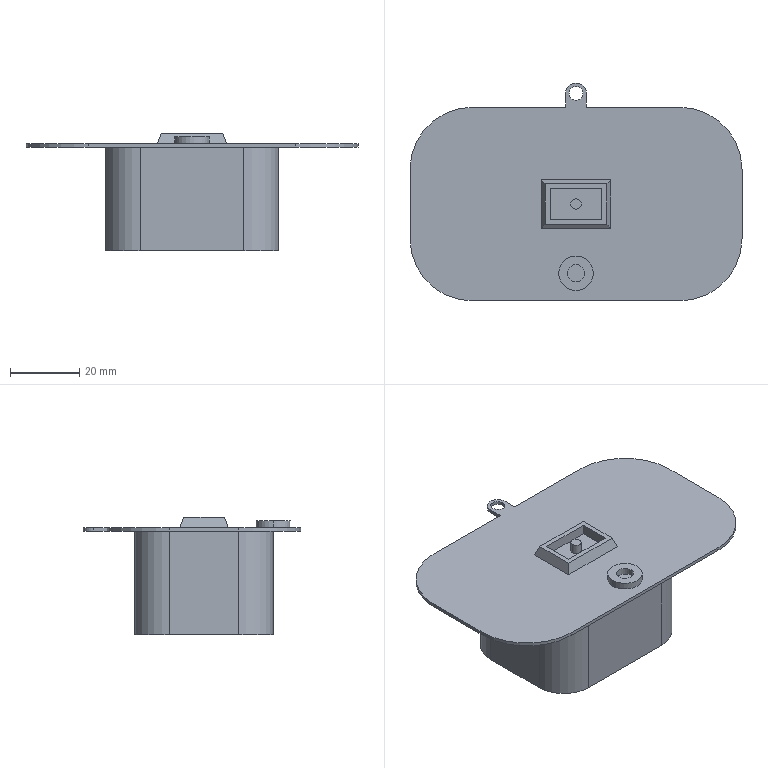Part | SolidWorks | features ICE 4, Fillet 2, Extrusion 1 | 1 solid | 53 faces | box 96 x 63 x 34 mm | volume 14984 mm3 | plane 32 | cylinder 21 | commonest cylinder face diameters 16 x4 20 x4 36 x4 3 x2 4 x2 5 x2
STEP:
#1=CARTESIAN_POINT('',(-2.5,-20.,3.));
#2=VERTEX_POINT('',#1);
#3=CARTESIAN_POINT('',(2.5,-20.,3.));
#4=VERTEX_POINT('',#3);
#5=CARTESIAN_POINT('',(0.,-20.,3.));
#6=DIRECTION('',(0.,0.,1.));
#7=DIRECTION('',(1.,0.,0.));
#8=AXIS2_PLACEMENT_3D('',#5,#6,#7);
#9=CIRCLE('',#8,2.5);
#10=EDGE_CURVE('',#2,#4,#9,.T.);
#11=ORIENTED_EDGE('',*,*,#10,.T.);
#12=CARTESIAN_POINT('',(2.5,-20.,1.));
#13=VERTEX_POINT('',#12);
#14=CARTESIAN_POINT('',(2.5,-20.,3.));
#15=DIRECTION('',(0.,0.,-1.));
#16=VECTOR('',#15,1000.);
#17=LINE('',#14,#16);
#18=EDGE_CURVE('',#4,#13,#17,.T.);
#19=ORIENTED_EDGE('',*,*,#18,.T.);
#20=CARTESIAN_POINT('',(-2.5,-20.,1.));
#21=VERTEX_POINT('',#20);
#22=CARTESIAN_POINT('',(0.,-20.,1.));
#23=DIRECTION('',(0.,0.,-1.));
#24=DIRECTION('',(1.,0.,0.));
#25=AXIS2_PLACEMENT_3D('',#22,#23,#24);
#26=CIRCLE('',#25,2.5);
#27=EDGE_CURVE('',#13,#21,#26,.T.);
#28=ORIENTED_EDGE('',*,*,#27,.T.);
#29=CARTESIAN_POINT('',(-2.5,-20.,3.));
#30=DIRECTION('',(0.,0.,-1.));
#31=VECTOR('',#30,1000.);
#32=LINE('',#29,#31);
#33=EDGE_CURVE('',#2,#21,#32,.T.);
#34=ORIENTED_EDGE('',*,*,#33,.F.);
#35=EDGE_LOOP('',(#11,#19,#28,#34));
#36=FACE_OUTER_BOUND('',#35,.T.);
#37=CARTESIAN_POINT('',(0.,-20.,3.));
#38=DIRECTION('',(0.,0.,-1.));
#39=DIRECTION('',(-1.,0.,0.));
#40=AXIS2_PLACEMENT_3D('',#37,#38,#39);
#41=CYLINDRICAL_SURFACE('',#40,2.5);
#42=ADVANCED_FACE('',(#36),#41,.F.);
#43=CARTESIAN_POINT('',(5.,-20.,3.));
#44=VERTEX_POINT('',#43);
#45=CARTESIAN_POINT('',(-5.,-20.,3.));
#46=VERTEX_POINT('',#45);
#47=CARTESIAN_POINT('',(0.,-20.,3.));
#48=DIRECTION('',(0.,0.,1.));
#49=DIRECTION('',(1.,0.,0.));
#50=AXIS2_PLACEMENT_3D('',#47,#48,#49);
#51=CIRCLE('',#50,5.);
#52=EDGE_CURVE('',#44,#46,#51,.T.);
#53=ORIENTED_EDGE('',*,*,#52,.F.);
#54=CARTESIAN_POINT('',(5.,-20.,1.));
#55=VERTEX_POINT('',#54);
#56=CARTESIAN_POINT('',(5.,-20.,3.));
#57=DIRECTION('',(0.,0.,-1.));
#58=VECTOR('',#57,1000.);
#59=LINE('',#56,#58);
#60=EDGE_CURVE('',#44,#55,#59,.T.);
#61=ORIENTED_EDGE('',*,*,#60,.T.);
#62=CARTESIAN_POINT('',(-5.,-20.,1.));
#63=VERTEX_POINT('',#62);
#64=CARTESIAN_POINT('',(0.,-20.,1.));
#65=DIRECTION('',(0.,0.,1.));
#66=DIRECTION('',(1.,0.,0.));
#67=AXIS2_PLACEMENT_3D('',#64,#65,#66);
#68=CIRCLE('',#67,5.);
#69=EDGE_CURVE('',#55,#63,#68,.T.);
#70=ORIENTED_EDGE('',*,*,#69,.T.);
#71=CARTESIAN_POINT('',(-5.,-20.,3.));
#72=DIRECTION('',(0.,0.,-1.));
#73=VECTOR('',#72,1000.);
#74=LINE('',#71,#73);
#75=EDGE_CURVE('',#46,#63,#74,.T.);
#76=ORIENTED_EDGE('',*,*,#75,.F.);
#77=EDGE_LOOP('',(#53,#61,#70,#76));
#78=FACE_OUTER_BOUND('',#77,.T.);
#79=CARTESIAN_POINT('',(0.,-20.,3.));
#80=DIRECTION('',(0.,0.,-1.));
#81=DIRECTION('',(-1.,0.,0.));
#82=AXIS2_PLACEMENT_3D('',#79,#80,#81);
#83=CYLINDRICAL_SURFACE('',#82,5.);
#84=ADVANCED_FACE('',(#78),#83,.T.);
#85=CARTESIAN_POINT('',(1.5,0.,1.));
#86=VERTEX_POINT('',#85);
#87=CARTESIAN_POINT('',(-1.5,0.,1.));
#88=VERTEX_POINT('',#87);
#89=CARTESIAN_POINT('',(0.,0.,1.));
#90=DIRECTION('',(0.,0.,1.));
#91=DIRECTION('',(1.,0.,0.));
#92=AXIS2_PLACEMENT_3D('',#89,#90,#91);
#93=CIRCLE('',#92,1.5);
#94=EDGE_CURVE('',#86,#88,#93,.T.);
#95=ORIENTED_EDGE('',*,*,#94,.T.);
#96=CARTESIAN_POINT('',(-1.5,0.,4.));
#97=VERTEX_POINT('',#96);
#98=CARTESIAN_POINT('',(-1.5,0.,1.));
#99=DIRECTION('',(0.,0.,1.));
#100=VECTOR('',#99,1000.);
#101=LINE('',#98,#100);
#102=EDGE_CURVE('',#88,#97,#101,.T.);
#103=ORIENTED_EDGE('',*,*,#102,.T.);
#104=CARTESIAN_POINT('',(1.5,0.,4.));
#105=VERTEX_POINT('',#104);
#106=CARTESIAN_POINT('',(0.,0.,4.));
#107=DIRECTION('',(0.,0.,1.));
#108=DIRECTION('',(1.,0.,0.));
#109=AXIS2_PLACEMENT_3D('',#106,#107,#108);
#110=CIRCLE('',#109,1.5);
#111=EDGE_CURVE('',#105,#97,#110,.T.);
#112=ORIENTED_EDGE('',*,*,#111,.F.);
#113=CARTESIAN_POINT('',(1.5,0.,1.));
#114=DIRECTION('',(0.,0.,1.));
#115=VECTOR('',#114,1000.);
#116=LINE('',#113,#115);
#117=EDGE_CURVE('',#86,#105,#116,.T.);
#118=ORIENTED_EDGE('',*,*,#117,.F.);
#119=EDGE_LOOP('',(#95,#103,#112,#118));
#120=FACE_OUTER_BOUND('',#119,.T.);
#121=CARTESIAN_POINT('',(0.,0.,1.));
#122=DIRECTION('',(0.,0.,1.));
#123=DIRECTION('',(1.,0.,0.));
#124=AXIS2_PLACEMENT_3D('',#121,#122,#123);
#125=CYLINDRICAL_SURFACE('',#124,1.5);
#126=ADVANCED_FACE('',(#120),#125,.T.);
#127=CARTESIAN_POINT('',(-2.,32.,1.));
#128=VERTEX_POINT('',#127);
#129=CARTESIAN_POINT('',(2.,32.,1.));
#130=VERTEX_POINT('',#129);
#131=CARTESIAN_POINT('',(0.,32.,1.));
#132=DIRECTION('',(0.,0.,1.));
#133=DIRECTION('',(1.,0.,0.));
#134=AXIS2_PLACEMENT_3D('',#131,#132,#133);
#135=CIRCLE('',#134,2.);
#136=EDGE_CURVE('',#128,#130,#135,.T.);
#137=ORIENTED_EDGE('',*,*,#136,.T.);
#138=CARTESIAN_POINT('',(2.,32.,0.));
#139=VERTEX_POINT('',#138);
#140=CARTESIAN_POINT('',(2.,32.,1.));
#141=DIRECTION('',(0.,0.,-1.));
#142=VECTOR('',#141,1000.);
#143=LINE('',#140,#142);
#144=EDGE_CURVE('',#130,#139,#143,.T.);
#145=ORIENTED_EDGE('',*,*,#144,.T.);
#146=CARTESIAN_POINT('',(-2.,32.,0.));
#147=VERTEX_POINT('',#146);
#148=CARTESIAN_POINT('',(0.,32.,0.));
#149=DIRECTION('',(0.,0.,1.));
#150=DIRECTION('',(1.,0.,0.));
#151=AXIS2_PLACEMENT_3D('',#148,#149,#150);
#152=CIRCLE('',#151,2.);
#153=EDGE_CURVE('',#147,#139,#152,.T.);
#154=ORIENTED_EDGE('',*,*,#153,.F.);
#155=CARTESIAN_POINT('',(-2.,32.,1.));
#156=DIRECTION('',(0.,0.,-1.));
#157=VECTOR('',#156,1000.);
#158=LINE('',#155,#157);
#159=EDGE_CURVE('',#128,#147,#158,.T.);
#160=ORIENTED_EDGE('',*,*,#159,.F.);
#161=EDGE_LOOP('',(#137,#145,#154,#160));
#162=FACE_OUTER_BOUND('',#161,.T.);
#163=CARTESIAN_POINT('',(0.,32.,1.));
#164=DIRECTION('',(0.,0.,-1.));
#165=DIRECTION('',(-1.,0.,0.));
#166=AXIS2_PLACEMENT_3D('',#163,#164,#165);
#167=CYLINDRICAL_SURFACE('',#166,2.);
#168=ADVANCED_FACE('',(#162),#167,.F.);
#169=CARTESIAN_POINT('',(-48.,-10.,0.));
#170=VERTEX_POINT('',#169);
#171=CARTESIAN_POINT('',(-30.,-28.,0.));
#172=VERTEX_POINT('',#171);
#173=CARTESIAN_POINT('',(-30.,-10.,0.));
#174=DIRECTION('',(0.,0.,1.));
#175=DIRECTION('',(1.,0.,0.));
#176=AXIS2_PLACEMENT_3D('',#173,#174,#175);
#177=CIRCLE('',#176,18.);
#178=EDGE_CURVE('',#170,#172,#177,.T.);
#179=ORIENTED_EDGE('',*,*,#178,.F.);
#180=CARTESIAN_POINT('',(-48.,10.,0.));
#181=VERTEX_POINT('',#180);
#182=CARTESIAN_POINT('',(-48.,10.,0.));
#183=DIRECTION('',(0.,-1.,0.));
#184=VECTOR('',#183,1000.);
#185=LINE('',#182,#184);
#186=EDGE_CURVE('',#181,#170,#185,.T.);
#187=ORIENTED_EDGE('',*,*,#186,.F.);
#188=CARTESIAN_POINT('',(-30.,28.,0.));
#189=VERTEX_POINT('',#188);
#190=CARTESIAN_POINT('',(-30.,10.,0.));
#191=DIRECTION('',(0.,0.,1.));
#192=DIRECTION('',(1.,0.,0.));
#193=AXIS2_PLACEMENT_3D('',#190,#191,#192);
#194=CIRCLE('',#193,18.);
#195=EDGE_CURVE('',#189,#181,#194,.T.);
#196=ORIENTED_EDGE('',*,*,#195,.F.);
#197=CARTESIAN_POINT('',(-3.,28.,0.));
#198=VERTEX_POINT('',#197);
#199=CARTESIAN_POINT('',(-30.,28.,0.));
#200=DIRECTION('',(-1.,0.,0.));
#201=VECTOR('',#200,1000.);
#202=LINE('',#199,#201);
#203=EDGE_CURVE('',#198,#189,#202,.T.);
#204=ORIENTED_EDGE('',*,*,#203,.F.);
#205=CARTESIAN_POINT('',(-3.,32.,0.));
#206=VERTEX_POINT('',#205);
#207=CARTESIAN_POINT('',(-3.,28.,0.));
#208=DIRECTION('',(0.,-1.,0.));
#209=VECTOR('',#208,1000.);
#210=LINE('',#207,#209);
#211=EDGE_CURVE('',#206,#198,#210,.T.);
#212=ORIENTED_EDGE('',*,*,#211,.F.);
#213=CARTESIAN_POINT('',(3.,32.,0.));
#214=VERTEX_POINT('',#213);
#215=CARTESIAN_POINT('',(0.,32.,0.));
#216=DIRECTION('',(0.,0.,1.));
#217=DIRECTION('',(-1.,0.,0.));
#218=AXIS2_PLACEMENT_3D('',#215,#216,#217);
#219=CIRCLE('',#218,3.);
#220=EDGE_CURVE('',#214,#206,#219,.T.);
#221=ORIENTED_EDGE('',*,*,#220,.F.);
#222=CARTESIAN_POINT('',(3.,28.,0.));
#223=VERTEX_POINT('',#222);
#224=CARTESIAN_POINT('',(3.,32.,0.));
#225=DIRECTION('',(0.,1.,0.));
#226=VECTOR('',#225,1000.);
#227=LINE('',#224,#226);
#228=EDGE_CURVE('',#223,#214,#227,.T.);
#229=ORIENTED_EDGE('',*,*,#228,.F.);
#230=CARTESIAN_POINT('',(30.,28.,0.));
#231=VERTEX_POINT('',#230);
#232=CARTESIAN_POINT('',(3.,28.,0.));
#233=DIRECTION('',(-1.,0.,0.));
#234=VECTOR('',#233,1000.);
#235=LINE('',#232,#234);
#236=EDGE_CURVE('',#231,#223,#235,.T.);
#237=ORIENTED_EDGE('',*,*,#236,.F.);
#238=CARTESIAN_POINT('',(48.,10.,0.));
#239=VERTEX_POINT('',#238);
#240=CARTESIAN_POINT('',(30.,10.,0.));
#241=DIRECTION('',(0.,0.,1.));
#242=DIRECTION('',(-1.,0.,0.));
#243=AXIS2_PLACEMENT_3D('',#240,#241,#242);
#244=CIRCLE('',#243,18.);
#245=EDGE_CURVE('',#239,#231,#244,.T.);
#246=ORIENTED_EDGE('',*,*,#245,.F.);
#247=CARTESIAN_POINT('',(48.,-10.,0.));
#248=VERTEX_POINT('',#247);
#249=CARTESIAN_POINT('',(48.,10.,0.));
#250=DIRECTION('',(0.,1.,0.));
#251=VECTOR('',#250,1000.);
#252=LINE('',#249,#251);
#253=EDGE_CURVE('',#248,#239,#252,.T.);
#254=ORIENTED_EDGE('',*,*,#253,.F.);
#255=CARTESIAN_POINT('',(30.,-28.,0.));
#256=VERTEX_POINT('',#255);
#257=CARTESIAN_POINT('',(30.,-10.,0.));
#258=DIRECTION('',(0.,0.,1.));
#259=DIRECTION('',(1.,0.,0.));
#260=AXIS2_PLACEMENT_3D('',#257,#258,#259);
#261=CIRCLE('',#260,18.);
#262=EDGE_CURVE('',#256,#248,#261,.T.);
#263=ORIENTED_EDGE('',*,*,#262,.F.);
#264=CARTESIAN_POINT('',(-30.,-28.,0.));
#265=DIRECTION('',(1.,0.,0.));
#266=VECTOR('',#265,1000.);
#267=LINE('',#264,#266);
#268=EDGE_CURVE('',#172,#256,#267,.T.);
#269=ORIENTED_EDGE('',*,*,#268,.F.);
#270=EDGE_LOOP('',(#179,#187,#196,#204,#212,#221,#229,#237,#246,#254,#263,#269));
#271=FACE_OUTER_BOUND('',#270,.T.);
#272=ORIENTED_EDGE('',*,*,#153,.T.);
#273=CARTESIAN_POINT('',(0.,32.,0.));
#274=DIRECTION('',(0.,0.,1.));
#275=DIRECTION('',(1.,0.,0.));
#276=AXIS2_PLACEMENT_3D('',#273,#274,#275);
#277=CIRCLE('',#276,2.);
#278=EDGE_CURVE('',#139,#147,#277,.T.);
#279=ORIENTED_EDGE('',*,*,#278,.T.);
#280=EDGE_LOOP('',(#272,#279));
#281=FACE_BOUND('',#280,.T.);
#282=CARTESIAN_POINT('',(-25.,-10.,0.));
#283=VERTEX_POINT('',#282);
#284=CARTESIAN_POINT('',(-25.,10.,0.));
#285=VERTEX_POINT('',#284);
#286=CARTESIAN_POINT('',(-25.,20.,0.));
#287=DIRECTION('',(0.,1.,0.));
#288=VECTOR('',#287,1000.);
#289=LINE('',#286,#288);
#290=EDGE_CURVE('',#283,#285,#289,.T.);
#291=ORIENTED_EDGE('',*,*,#290,.F.);
#292=CARTESIAN_POINT('',(-15.,-20.,0.));
#293=VERTEX_POINT('',#292);
#294=CARTESIAN_POINT('',(-15.,-10.,0.));
#295=DIRECTION('',(0.,0.,1.));
#296=DIRECTION('',(1.,0.,0.));
#297=AXIS2_PLACEMENT_3D('',#294,#295,#296);
#298=CIRCLE('',#297,10.);
#299=EDGE_CURVE('',#283,#293,#298,.T.);
#300=ORIENTED_EDGE('',*,*,#299,.T.);
#301=CARTESIAN_POINT('',(15.,-20.,0.));
#302=VERTEX_POINT('',#301);
#303=CARTESIAN_POINT('',(25.,-20.,0.));
#304=DIRECTION('',(-1.,0.,0.));
#305=VECTOR('',#304,1000.);
#306=LINE('',#303,#305);
#307=EDGE_CURVE('',#302,#293,#306,.T.);
#308=ORIENTED_EDGE('',*,*,#307,.F.);
#309=CARTESIAN_POINT('',(25.,-10.,0.));
#310=VERTEX_POINT('',#309);
#311=CARTESIAN_POINT('',(15.,-10.,0.));
#312=DIRECTION('',(0.,0.,1.));
#313=DIRECTION('',(1.,0.,0.));
#314=AXIS2_PLACEMENT_3D('',#311,#312,#313);
#315=CIRCLE('',#314,10.);
#316=EDGE_CURVE('',#302,#310,#315,.T.);
#317=ORIENTED_EDGE('',*,*,#316,.T.);
#318=CARTESIAN_POINT('',(25.,10.,0.));
#319=VERTEX_POINT('',#318);
#320=CARTESIAN_POINT('',(25.,20.,0.));
#321=DIRECTION('',(0.,-1.,0.));
#322=VECTOR('',#321,1000.);
#323=LINE('',#320,#322);
#324=EDGE_CURVE('',#319,#310,#323,.T.);
#325=ORIENTED_EDGE('',*,*,#324,.F.);
#326=CARTESIAN_POINT('',(15.,20.,0.));
#327=VERTEX_POINT('',#326);
#328=CARTESIAN_POINT('',(15.,10.,0.));
#329=DIRECTION('',(0.,0.,1.));
#330=DIRECTION('',(1.,0.,0.));
#331=AXIS2_PLACEMENT_3D('',#328,#329,#330);
#332=CIRCLE('',#331,10.);
#333=EDGE_CURVE('',#319,#327,#332,.T.);
#334=ORIENTED_EDGE('',*,*,#333,.T.);
#335=CARTESIAN_POINT('',(-15.,20.,0.));
#336=VERTEX_POINT('',#335);
#337=CARTESIAN_POINT('',(25.,20.,0.));
#338=DIRECTION('',(1.,0.,0.));
#339=VECTOR('',#338,1000.);
#340=LINE('',#337,#339);
#341=EDGE_CURVE('',#336,#327,#340,.T.);
#342=ORIENTED_EDGE('',*,*,#341,.F.);
#343=CARTESIAN_POINT('',(-15.,10.,0.));
#344=DIRECTION('',(0.,0.,1.));
#345=DIRECTION('',(1.,0.,0.));
#346=AXIS2_PLACEMENT_3D('',#343,#344,#345);
#347=CIRCLE('',#346,10.);
#348=EDGE_CURVE('',#336,#285,#347,.T.);
#349=ORIENTED_EDGE('',*,*,#348,.T.);
#350=EDGE_LOOP('',(#291,#300,#308,#317,#325,#334,#342,#349));
#351=FACE_BOUND('',#350,.T.);
#352=CARTESIAN_POINT('',(-30.,-10.,0.));
#353=DIRECTION('',(0.,0.,1.));
#354=DIRECTION('',(1.,0.,0.));
#355=AXIS2_PLACEMENT_3D('',#352,#353,#354);
#356=PLANE('',#355);
#357=ADVANCED_FACE('',(#271,#281,#351),#356,.F.);
#358=CARTESIAN_POINT('',(0.,-20.,1.));
#359=DIRECTION('',(0.,0.,1.));
#360=DIRECTION('',(1.,0.,0.));
#361=AXIS2_PLACEMENT_3D('',#358,#359,#360);
#362=CIRCLE('',#361,5.);
#363=EDGE_CURVE('',#63,#55,#362,.T.);
#364=ORIENTED_EDGE('',*,*,#363,.F.);
#365=ORIENTED_EDGE('',*,*,#69,.F.);
#366=EDGE_LOOP('',(#364,#365));
#367=FACE_BOUND('',#366,.T.);
#368=CARTESIAN_POINT('',(-48.,-10.,1.));
#369=VERTEX_POINT('',#368);
#370=CARTESIAN_POINT('',(-30.,-28.,1.));
#371=VERTEX_POINT('',#370);
#372=CARTESIAN_POINT('',(-30.,-10.,1.));
#373=DIRECTION('',(0.,0.,1.));
#374=DIRECTION('',(1.,0.,0.));
#375=AXIS2_PLACEMENT_3D('',#372,#373,#374);
#376=CIRCLE('',#375,18.);
#377=EDGE_CURVE('',#369,#371,#376,.T.);
#378=ORIENTED_EDGE('',*,*,#377,.T.);
#379=CARTESIAN_POINT('',(30.,-28.,1.));
#380=VERTEX_POINT('',#379);
#381=CARTESIAN_POINT('',(-30.,-28.,1.));
#382=DIRECTION('',(1.,0.,0.));
#383=VECTOR('',#382,1000.);
#384=LINE('',#381,#383);
#385=EDGE_CURVE('',#371,#380,#384,.T.);
#386=ORIENTED_EDGE('',*,*,#385,.T.);
#387=CARTESIAN_POINT('',(48.,-10.,1.));
#388=VERTEX_POINT('',#387);
#389=CARTESIAN_POINT('',(30.,-10.,1.));
#390=DIRECTION('',(0.,0.,1.));
#391=DIRECTION('',(1.,0.,0.));
#392=AXIS2_PLACEMENT_3D('',#389,#390,#391);
#393=CIRCLE('',#392,18.);
#394=EDGE_CURVE('',#380,#388,#393,.T.);
#395=ORIENTED_EDGE('',*,*,#394,.T.);
#396=CARTESIAN_POINT('',(48.,10.,1.));
#397=VERTEX_POINT('',#396);
#398=CARTESIAN_POINT('',(48.,10.,1.));
#399=DIRECTION('',(0.,1.,0.));
#400=VECTOR('',#399,1000.);
#401=LINE('',#398,#400);
#402=EDGE_CURVE('',#388,#397,#401,.T.);
#403=ORIENTED_EDGE('',*,*,#402,.T.);
#404=CARTESIAN_POINT('',(30.,28.,1.));
#405=VERTEX_POINT('',#404);
#406=CARTESIAN_POINT('',(30.,10.,1.));
#407=DIRECTION('',(0.,0.,1.));
#408=DIRECTION('',(-1.,0.,0.));
#409=AXIS2_PLACEMENT_3D('',#406,#407,#408);
#410=CIRCLE('',#409,18.);
#411=EDGE_CURVE('',#397,#405,#410,.T.);
#412=ORIENTED_EDGE('',*,*,#411,.T.);
#413=CARTESIAN_POINT('',(3.,28.,1.));
#414=VERTEX_POINT('',#413);
#415=CARTESIAN_POINT('',(3.,28.,1.));
#416=DIRECTION('',(-1.,0.,0.));
#417=VECTOR('',#416,1000.);
#418=LINE('',#415,#417);
#419=EDGE_CURVE('',#405,#414,#418,.T.);
#420=ORIENTED_EDGE('',*,*,#419,.T.);
#421=CARTESIAN_POINT('',(3.,32.,1.));
#422=VERTEX_POINT('',#421);
#423=CARTESIAN_POINT('',(3.,32.,1.));
#424=DIRECTION('',(0.,1.,0.));
#425=VECTOR('',#424,1000.);
#426=LINE('',#423,#425);
#427=EDGE_CURVE('',#414,#422,#426,.T.);
#428=ORIENTED_EDGE('',*,*,#427,.T.);
#429=CARTESIAN_POINT('',(-3.,32.,1.));
#430=VERTEX_POINT('',#429);
#431=CARTESIAN_POINT('',(0.,32.,1.));
#432=DIRECTION('',(0.,0.,1.));
#433=DIRECTION('',(-1.,0.,0.));
#434=AXIS2_PLACEMENT_3D('',#431,#432,#433);
#435=CIRCLE('',#434,3.);
#436=EDGE_CURVE('',#422,#430,#435,.T.);
#437=ORIENTED_EDGE('',*,*,#436,.T.);
#438=CARTESIAN_POINT('',(-3.,28.,1.));
#439=VERTEX_POINT('',#438);
#440=CARTESIAN_POINT('',(-3.,28.,1.));
#441=DIRECTION('',(0.,-1.,0.));
#442=VECTOR('',#441,1000.);
#443=LINE('',#440,#442);
#444=EDGE_CURVE('',#430,#439,#443,.T.);
#445=ORIENTED_EDGE('',*,*,#444,.T.);
#446=CARTESIAN_POINT('',(-30.,28.,1.));
#447=VERTEX_POINT('',#446);
#448=CARTESIAN_POINT('',(-30.,28.,1.));
#449=DIRECTION('',(-1.,0.,0.));
#450=VECTOR('',#449,1000.);
#451=LINE('',#448,#450);
#452=EDGE_CURVE('',#439,#447,#451,.T.);
#453=ORIENTED_EDGE('',*,*,#452,.T.);
#454=CARTESIAN_POINT('',(-48.,10.,1.));
#455=VERTEX_POINT('',#454);
#456=CARTESIAN_POINT('',(-30.,10.,1.));
#457=DIRECTION('',(0.,0.,1.));
#458=DIRECTION('',(1.,0.,0.));
#459=AXIS2_PLACEMENT_3D('',#456,#457,#458);
#460=CIRCLE('',#459,18.);
#461=EDGE_CURVE('',#447,#455,#460,.T.);
#462=ORIENTED_EDGE('',*,*,#461,.T.);
#463=CARTESIAN_POINT('',(-48.,10.,1.));
#464=DIRECTION('',(0.,-1.,0.));
#465=VECTOR('',#464,1000.);
#466=LINE('',#463,#465);
#467=EDGE_CURVE('',#455,#369,#466,.T.);
#468=ORIENTED_EDGE('',*,*,#467,.T.);
#469=EDGE_LOOP('',(#378,#386,#395,#403,#412,#420,#428,#437,#445,#453,#462,#468));
#470=FACE_OUTER_BOUND('',#469,.T.);
#471=ORIENTED_EDGE('',*,*,#136,.F.);
#472=CARTESIAN_POINT('',(0.,32.,1.));
#473=DIRECTION('',(0.,0.,1.));
#474=DIRECTION('',(1.,0.,0.));
#475=AXIS2_PLACEMENT_3D('',#472,#473,#474);
#476=CIRCLE('',#475,2.);
#477=EDGE_CURVE('',#130,#128,#476,.T.);
#478=ORIENTED_EDGE('',*,*,#477,.F.);
#479=EDGE_LOOP('',(#471,#478));
#480=FACE_BOUND('',#479,.T.);
#481=CARTESIAN_POINT('',(10.,7.,1.));
#482=VERTEX_POINT('',#481);
#483=CARTESIAN_POINT('',(-10.,7.,1.));
#484=VERTEX_POINT('',#483);
#485=CARTESIAN_POINT('',(-10.,7.,1.));
#486=DIRECTION('',(-1.,0.,0.));
#487=VECTOR('',#486,1000.);
#488=LINE('',#485,#487);
#489=EDGE_CURVE('',#482,#484,#488,.T.);
#490=ORIENTED_EDGE('',*,*,#489,.F.);
#491=CARTESIAN_POINT('',(10.,-7.,1.));
#492=VERTEX_POINT('',#491);
#493=CARTESIAN_POINT('',(10.,7.,1.));
#494=DIRECTION('',(0.,1.,0.));
#495=VECTOR('',#494,1000.);
#496=LINE('',#493,#495);
#497=EDGE_CURVE('',#492,#482,#496,.T.);
#498=ORIENTED_EDGE('',*,*,#497,.F.);
#499=CARTESIAN_POINT('',(-10.,-7.,1.));
#500=VERTEX_POINT('',#499);
#501=CARTESIAN_POINT('',(-10.,-7.,1.));
#502=DIRECTION('',(1.,0.,0.));
#503=VECTOR('',#502,1000.);
#504=LINE('',#501,#503);
#505=EDGE_CURVE('',#500,#492,#504,.T.);
#506=ORIENTED_EDGE('',*,*,#505,.F.);
#507=CARTESIAN_POINT('',(-10.,7.,1.));
#508=DIRECTION('',(0.,-1.,0.));
#509=VECTOR('',#508,1000.);
#510=LINE('',#507,#509);
#511=EDGE_CURVE('',#484,#500,#510,.T.);
#512=ORIENTED_EDGE('',*,*,#511,.F.);
#513=EDGE_LOOP('',(#490,#498,#506,#512));
#514=FACE_BOUND('',#513,.T.);
#515=CARTESIAN_POINT('',(-30.,-10.,1.));
#516=DIRECTION('',(0.,0.,1.));
#517=DIRECTION('',(1.,0.,0.));
#518=AXIS2_PLACEMENT_3D('',#515,#516,#517);
#519=PLANE('',#518);
#520=ADVANCED_FACE('',(#367,#470,#480,#514),#519,.T.);
#521=ORIENTED_EDGE('',*,*,#178,.T.);
#522=CARTESIAN_POINT('',(-30.,-28.,1.));
#523=DIRECTION('',(0.,0.,-1.));
#524=VECTOR('',#523,1000.);
#525=LINE('',#522,#524);
#526=EDGE_CURVE('',#371,#172,#525,.T.);
#527=ORIENTED_EDGE('',*,*,#526,.F.);
#528=ORIENTED_EDGE('',*,*,#377,.F.);
#529=CARTESIAN_POINT('',(-48.,-10.,1.));
#530=DIRECTION('',(0.,0.,-1.));
#531=VECTOR('',#530,1000.);
#532=LINE('',#529,#531);
#533=EDGE_CURVE('',#369,#170,#532,.T.);
#534=ORIENTED_EDGE('',*,*,#533,.T.);
#535=EDGE_LOOP('',(#521,#527,#528,#534));
#536=FACE_OUTER_BOUND('',#535,.T.);
#537=CARTESIAN_POINT('',(-30.,-10.,1.));
#538=DIRECTION('',(0.,0.,-1.));
#539=DIRECTION('',(-1.,0.,0.));
#540=AXIS2_PLACEMENT_3D('',#537,#538,#539);
#541=CYLINDRICAL_SURFACE('',#540,18.);
#542=ADVANCED_FACE('',(#536),#541,.T.);
#543=ORIENTED_EDGE('',*,*,#268,.T.);
#544=CARTESIAN_POINT('',(30.,-28.,1.));
#545=DIRECTION('',(0.,0.,-1.));
#546=VECTOR('',#545,1000.);
#547=LINE('',#544,#546);
#548=EDGE_CURVE('',#380,#256,#547,.T.);
#549=ORIENTED_EDGE('',*,*,#548,.F.);
#550=ORIENTED_EDGE('',*,*,#385,.F.);
#551=ORIENTED_EDGE('',*,*,#526,.T.);
#552=EDGE_LOOP('',(#543,#549,#550,#551));
#553=FACE_OUTER_BOUND('',#552,.T.);
#554=CARTESIAN_POINT('',(-30.,-28.,1.));
#555=DIRECTION('',(0.,1.,0.));
#556=DIRECTION('',(0.,0.,1.));
#557=AXIS2_PLACEMENT_3D('',#554,#555,#556);
#558=PLANE('',#557);
#559=ADVANCED_FACE('',(#553),#558,.F.);
#560=ORIENTED_EDGE('',*,*,#262,.T.);
#561=CARTESIAN_POINT('',(48.,-10.,1.));
#562=DIRECTION('',(0.,0.,-1.));
#563=VECTOR('',#562,1000.);
#564=LINE('',#561,#563);
#565=EDGE_CURVE('',#388,#248,#564,.T.);
#566=ORIENTED_EDGE('',*,*,#565,.F.);
#567=ORIENTED_EDGE('',*,*,#394,.F.);
#568=ORIENTED_EDGE('',*,*,#548,.T.);
#569=EDGE_LOOP('',(#560,#566,#567,#568));
#570=FACE_OUTER_BOUND('',#569,.T.);
#571=CARTESIAN_POINT('',(30.,-10.,1.));
#572=DIRECTION('',(0.,0.,-1.));
#573=DIRECTION('',(-1.,0.,0.));
#574=AXIS2_PLACEMENT_3D('',#571,#572,#573);
#575=CYLINDRICAL_SURFACE('',#574,18.);
#576=ADVANCED_FACE('',(#570),#575,.T.);
#577=ORIENTED_EDGE('',*,*,#253,.T.);
#578=CARTESIAN_POINT('',(48.,10.,1.));
#579=DIRECTION('',(0.,0.,-1.));
#580=VECTOR('',#579,1000.);
#581=LINE('',#578,#580);
#582=EDGE_CURVE('',#397,#239,#581,.T.);
#583=ORIENTED_EDGE('',*,*,#582,.F.);
#584=ORIENTED_EDGE('',*,*,#402,.F.);
#585=ORIENTED_EDGE('',*,*,#565,.T.);
#586=EDGE_LOOP('',(#577,#583,#584,#585));
#587=FACE_OUTER_BOUND('',#586,.T.);
#588=CARTESIAN_POINT('',(48.,10.,1.));
#589=DIRECTION('',(-1.,0.,0.));
#590=DIRECTION('',(0.,0.,1.));
#591=AXIS2_PLACEMENT_3D('',#588,#589,#590);
#592=PLANE('',#591);
#593=ADVANCED_FACE('',(#587),#592,.F.);
#594=ORIENTED_EDGE('',*,*,#245,.T.);
#595=CARTESIAN_POINT('',(30.,28.,1.));
#596=DIRECTION('',(0.,0.,-1.));
#597=VECTOR('',#596,1000.);
#598=LINE('',#595,#597);
#599=EDGE_CURVE('',#405,#231,#598,.T.);
#600=ORIENTED_EDGE('',*,*,#599,.F.);
#601=ORIENTED_EDGE('',*,*,#411,.F.);
#602=ORIENTED_EDGE('',*,*,#582,.T.);
#603=EDGE_LOOP('',(#594,#600,#601,#602));
#604=FACE_OUTER_BOUND('',#603,.T.);
#605=CARTESIAN_POINT('',(30.,10.,1.));
#606=DIRECTION('',(0.,0.,-1.));
#607=DIRECTION('',(-1.,0.,0.));
#608=AXIS2_PLACEMENT_3D('',#605,#606,#607);
#609=CYLINDRICAL_SURFACE('',#608,18.);
#610=ADVANCED_FACE('',(#604),#609,.T.);
#611=ORIENTED_EDGE('',*,*,#236,.T.);
#612=CARTESIAN_POINT('',(3.,28.,1.));
#613=DIRECTION('',(0.,0.,-1.));
#614=VECTOR('',#613,1000.);
#615=LINE('',#612,#614);
#616=EDGE_CURVE('',#414,#223,#615,.T.);
#617=ORIENTED_EDGE('',*,*,#616,.F.);
#618=ORIENTED_EDGE('',*,*,#419,.F.);
#619=ORIENTED_EDGE('',*,*,#599,.T.);
#620=EDGE_LOOP('',(#611,#617,#618,#619));
#621=FACE_OUTER_BOUND('',#620,.T.);
#622=CARTESIAN_POINT('',(3.,28.,1.));
#623=DIRECTION('',(0.,-1.,0.));
#624=DIRECTION('',(0.,0.,-1.));
#625=AXIS2_PLACEMENT_3D('',#622,#623,#624);
#626=PLANE('',#625);
#627=ADVANCED_FACE('',(#621),#626,.F.);
#628=ORIENTED_EDGE('',*,*,#228,.T.);
#629=CARTESIAN_POINT('',(3.,32.,1.));
#630=DIRECTION('',(0.,0.,-1.));
#631=VECTOR('',#630,1000.);
#632=LINE('',#629,#631);
#633=EDGE_CURVE('',#422,#214,#632,.T.);
#634=ORIENTED_EDGE('',*,*,#633,.F.);
#635=ORIENTED_EDGE('',*,*,#427,.F.);
#636=ORIENTED_EDGE('',*,*,#616,.T.);
#637=EDGE_LOOP('',(#628,#634,#635,#636));
#638=FACE_OUTER_BOUND('',#637,.T.);
#639=CARTESIAN_POINT('',(3.,32.,1.));
#640=DIRECTION('',(-1.,0.,0.));
#641=DIRECTION('',(0.,0.,1.));
#642=AXIS2_PLACEMENT_3D('',#639,#640,#641);
#643=PLANE('',#642);
#644=ADVANCED_FACE('',(#638),#643,.F.);
#645=ORIENTED_EDGE('',*,*,#220,.T.);
#646=CARTESIAN_POINT('',(-3.,32.,1.));
#647=DIRECTION('',(0.,0.,-1.));
#648=VECTOR('',#647,1000.);
#649=LINE('',#646,#648);
#650=EDGE_CURVE('',#430,#206,#649,.T.);
#651=ORIENTED_EDGE('',*,*,#650,.F.);
#652=ORIENTED_EDGE('',*,*,#436,.F.);
#653=ORIENTED_EDGE('',*,*,#633,.T.);
#654=EDGE_LOOP('',(#645,#651,#652,#653));
#655=FACE_OUTER_BOUND('',#654,.T.);
#656=CARTESIAN_POINT('',(0.,32.,1.));
#657=DIRECTION('',(0.,0.,-1.));
#658=DIRECTION('',(-1.,0.,0.));
#659=AXIS2_PLACEMENT_3D('',#656,#657,#658);
#660=CYLINDRICAL_SURFACE('',#659,3.);
#661=ADVANCED_FACE('',(#655),#660,.T.);
#662=ORIENTED_EDGE('',*,*,#211,.T.);
#663=CARTESIAN_POINT('',(-3.,28.,1.));
#664=DIRECTION('',(0.,0.,-1.));
#665=VECTOR('',#664,1000.);
#666=LINE('',#663,#665);
#667=EDGE_CURVE('',#439,#198,#666,.T.);
#668=ORIENTED_EDGE('',*,*,#667,.F.);
#669=ORIENTED_EDGE('',*,*,#444,.F.);
#670=ORIENTED_EDGE('',*,*,#650,.T.);
#671=EDGE_LOOP('',(#662,#668,#669,#670));
#672=FACE_OUTER_BOUND('',#671,.T.);
#673=CARTESIAN_POINT('',(-3.,28.,1.));
#674=DIRECTION('',(1.,0.,0.));
#675=DIRECTION('',(0.,1.,0.));
#676=AXIS2_PLACEMENT_3D('',#673,#674,#675);
#677=PLANE('',#676);
#678=ADVANCED_FACE('',(#672),#677,.F.);
#679=ORIENTED_EDGE('',*,*,#203,.T.);
#680=CARTESIAN_POINT('',(-30.,28.,1.));
#681=DIRECTION('',(0.,0.,-1.));
#682=VECTOR('',#681,1000.);
#683=LINE('',#680,#682);
#684=EDGE_CURVE('',#447,#189,#683,.T.);
#685=ORIENTED_EDGE('',*,*,#684,.F.);
#686=ORIENTED_EDGE('',*,*,#452,.F.);
#687=ORIENTED_EDGE('',*,*,#667,.T.);
#688=EDGE_LOOP('',(#679,#685,#686,#687));
#689=FACE_OUTER_BOUND('',#688,.T.);
#690=CARTESIAN_POINT('',(-30.,28.,1.));
#691=DIRECTION('',(0.,-1.,0.));
#692=DIRECTION('',(1.,0.,0.));
#693=AXIS2_PLACEMENT_3D('',#690,#691,#692);
#694=PLANE('',#693);
#695=ADVANCED_FACE('',(#689),#694,.F.);
#696=ORIENTED_EDGE('',*,*,#195,.T.);
#697=CARTESIAN_POINT('',(-48.,10.,1.));
#698=DIRECTION('',(0.,0.,-1.));
#699=VECTOR('',#698,1000.);
#700=LINE('',#697,#699);
#701=EDGE_CURVE('',#455,#181,#700,.T.);
#702=ORIENTED_EDGE('',*,*,#701,.F.);
#703=ORIENTED_EDGE('',*,*,#461,.F.);
#704=ORIENTED_EDGE('',*,*,#684,.T.);
#705=EDGE_LOOP('',(#696,#702,#703,#704));
#706=FACE_OUTER_BOUND('',#705,.T.);
#707=CARTESIAN_POINT('',(-30.,10.,1.));
#708=DIRECTION('',(0.,0.,-1.));
#709=DIRECTION('',(-1.,0.,0.));
#710=AXIS2_PLACEMENT_3D('',#707,#708,#709);
#711=CYLINDRICAL_SURFACE('',#710,18.);
#712=ADVANCED_FACE('',(#706),#711,.T.);
#713=ORIENTED_EDGE('',*,*,#186,.T.);
#714=ORIENTED_EDGE('',*,*,#533,.F.);
#715=ORIENTED_EDGE('',*,*,#467,.F.);
#716=ORIENTED_EDGE('',*,*,#701,.T.);
#717=EDGE_LOOP('',(#713,#714,#715,#716));
#718=FACE_OUTER_BOUND('',#717,.T.);
#719=CARTESIAN_POINT('',(-48.,10.,1.));
#720=DIRECTION('',(1.,0.,0.));
#721=DIRECTION('',(0.,0.,-1.));
#722=AXIS2_PLACEMENT_3D('',#719,#720,#721);
#723=PLANE('',#722);
#724=ADVANCED_FACE('',(#718),#723,.F.);
#725=ORIENTED_EDGE('',*,*,#144,.F.);
#726=ORIENTED_EDGE('',*,*,#477,.T.);
#727=ORIENTED_EDGE('',*,*,#159,.T.);
#728=ORIENTED_EDGE('',*,*,#278,.F.);
#729=EDGE_LOOP('',(#725,#726,#727,#728));
#730=FACE_OUTER_BOUND('',#729,.T.);
#731=CARTESIAN_POINT('',(0.,32.,1.));
#732=DIRECTION('',(0.,0.,-1.));
#733=DIRECTION('',(-1.,0.,0.));
#734=AXIS2_PLACEMENT_3D('',#731,#732,#733);
#735=CYLINDRICAL_SURFACE('',#734,2.);
#736=ADVANCED_FACE('',(#730),#735,.F.);
#737=ORIENTED_EDGE('',*,*,#497,.T.);
#738=CARTESIAN_POINT('',(8.908,5.908,4.));
#739=VERTEX_POINT('',#738);
#740=CARTESIAN_POINT('',(7.905,4.905,6.755));
#741=DIRECTION('',(0.3236,0.3236,-0.8891));
#742=VECTOR('',#741,1000.);
#743=LINE('',#740,#742);
#744=EDGE_CURVE('',#739,#482,#743,.T.);
#745=ORIENTED_EDGE('',*,*,#744,.F.);
#746=CARTESIAN_POINT('',(8.908,-5.908,4.));
#747=VERTEX_POINT('',#746);
#748=CARTESIAN_POINT('',(8.908,7.,4.));
#749=DIRECTION('',(0.,1.,0.));
#750=VECTOR('',#749,1000.);
#751=LINE('',#748,#750);
#752=EDGE_CURVE('',#747,#739,#751,.T.);
#753=ORIENTED_EDGE('',*,*,#752,.F.);
#754=CARTESIAN_POINT('',(8.534,-5.534,5.028));
#755=DIRECTION('',(0.3236,-0.3236,-0.8891));
#756=VECTOR('',#755,1000.);
#757=LINE('',#754,#756);
#758=EDGE_CURVE('',#747,#492,#757,.T.);
#759=ORIENTED_EDGE('',*,*,#758,.T.);
#760=EDGE_LOOP('',(#737,#745,#753,#759));
#761=FACE_OUTER_BOUND('',#760,.T.);
#762=CARTESIAN_POINT('',(10.,7.,1.));
#763=DIRECTION('',(0.9397,0.,0.342));
#764=DIRECTION('',(0.342,0.,-0.9397));
#765=AXIS2_PLACEMENT_3D('',#762,#763,#764);
#766=PLANE('',#765);
#767=ADVANCED_FACE('',(#761),#766,.T.);
#768=ORIENTED_EDGE('',*,*,#489,.T.);
#769=CARTESIAN_POINT('',(-8.908,5.908,4.));
#770=VERTEX_POINT('',#769);
#771=CARTESIAN_POINT('',(-10.,7.,1.));
#772=DIRECTION('',(-0.3236,0.3236,-0.8891));
#773=VECTOR('',#772,1000.);
#774=LINE('',#771,#773);
#775=EDGE_CURVE('',#770,#484,#774,.T.);
#776=ORIENTED_EDGE('',*,*,#775,.F.);
#777=CARTESIAN_POINT('',(-10.,5.908,4.));
#778=DIRECTION('',(-1.,0.,0.));
#779=VECTOR('',#778,1000.);
#780=LINE('',#777,#779);
#781=EDGE_CURVE('',#739,#770,#780,.T.);
#782=ORIENTED_EDGE('',*,*,#781,.F.);
#783=ORIENTED_EDGE('',*,*,#744,.T.);
#784=EDGE_LOOP('',(#768,#776,#782,#783));
#785=FACE_OUTER_BOUND('',#784,.T.);
#786=CARTESIAN_POINT('',(-10.,7.,1.));
#787=DIRECTION('',(0.,0.9397,0.342));
#788=DIRECTION('',(0.,-0.342,0.9397));
#789=AXIS2_PLACEMENT_3D('',#786,#787,#788);
#790=PLANE('',#789);
#791=ADVANCED_FACE('',(#785),#790,.T.);
#792=ORIENTED_EDGE('',*,*,#511,.T.);
#793=CARTESIAN_POINT('',(-8.908,-5.908,4.));
#794=VERTEX_POINT('',#793);
#795=CARTESIAN_POINT('',(-10.,-7.,1.));
#796=DIRECTION('',(-0.3236,-0.3236,-0.8891));
#797=VECTOR('',#796,1000.);
#798=LINE('',#795,#797);
#799=EDGE_CURVE('',#794,#500,#798,.T.);
#800=ORIENTED_EDGE('',*,*,#799,.F.);
#801=CARTESIAN_POINT('',(-8.908,7.,4.));
#802=DIRECTION('',(0.,-1.,0.));
#803=VECTOR('',#802,1000.);
#804=LINE('',#801,#803);
#805=EDGE_CURVE('',#770,#794,#804,.T.);
#806=ORIENTED_EDGE('',*,*,#805,.F.);
#807=ORIENTED_EDGE('',*,*,#775,.T.);
#808=EDGE_LOOP('',(#792,#800,#806,#807));
#809=FACE_OUTER_BOUND('',#808,.T.);
#810=CARTESIAN_POINT('',(-10.,7.,1.));
#811=DIRECTION('',(-0.9397,0.,0.342));
#812=DIRECTION('',(0.342,0.,0.9397));
#813=AXIS2_PLACEMENT_3D('',#810,#811,#812);
#814=PLANE('',#813);
#815=ADVANCED_FACE('',(#809),#814,.T.);
#816=ORIENTED_EDGE('',*,*,#505,.T.);
#817=ORIENTED_EDGE('',*,*,#758,.F.);
#818=CARTESIAN_POINT('',(-10.,-5.908,4.));
#819=DIRECTION('',(1.,0.,0.));
#820=VECTOR('',#819,1000.);
#821=LINE('',#818,#820);
#822=EDGE_CURVE('',#794,#747,#821,.T.);
#823=ORIENTED_EDGE('',*,*,#822,.F.);
#824=ORIENTED_EDGE('',*,*,#799,.T.);
#825=EDGE_LOOP('',(#816,#817,#823,#824));
#826=FACE_OUTER_BOUND('',#825,.T.);
#827=CARTESIAN_POINT('',(-10.,-7.,1.));
#828=DIRECTION('',(0.,-0.9397,0.342));
#829=DIRECTION('',(0.,-0.342,-0.9397));
#830=AXIS2_PLACEMENT_3D('',#827,#828,#829);
#831=PLANE('',#830);
#832=ADVANCED_FACE('',(#826),#831,.T.);
#833=CARTESIAN_POINT('',(7.5,-4.5,4.));
#834=VERTEX_POINT('',#833);
#835=CARTESIAN_POINT('',(7.5,4.5,4.));
#836=VERTEX_POINT('',#835);
#837=CARTESIAN_POINT('',(7.5,4.5,4.));
#838=DIRECTION('',(0.,1.,0.));
#839=VECTOR('',#838,1000.);
#840=LINE('',#837,#839);
#841=EDGE_CURVE('',#834,#836,#840,.T.);
#842=ORIENTED_EDGE('',*,*,#841,.F.);
#843=CARTESIAN_POINT('',(-7.5,-4.5,4.));
#844=VERTEX_POINT('',#843);
#845=CARTESIAN_POINT('',(-7.5,-4.5,4.));
#846=DIRECTION('',(1.,0.,0.));
#847=VECTOR('',#846,1000.);
#848=LINE('',#845,#847);
#849=EDGE_CURVE('',#844,#834,#848,.T.);
#850=ORIENTED_EDGE('',*,*,#849,.F.);
#851=CARTESIAN_POINT('',(-7.5,4.5,4.));
#852=VERTEX_POINT('',#851);
#853=CARTESIAN_POINT('',(-7.5,4.5,4.));
#854=DIRECTION('',(0.,-1.,0.));
#855=VECTOR('',#854,1000.);
#856=LINE('',#853,#855);
#857=EDGE_CURVE('',#852,#844,#856,.T.);
#858=ORIENTED_EDGE('',*,*,#857,.F.);
#859=CARTESIAN_POINT('',(-7.5,4.5,4.));
#860=DIRECTION('',(-1.,0.,0.));
#861=VECTOR('',#860,1000.);
#862=LINE('',#859,#861);
#863=EDGE_CURVE('',#836,#852,#862,.T.);
#864=ORIENTED_EDGE('',*,*,#863,.F.);
#865=EDGE_LOOP('',(#842,#850,#858,#864));
#866=FACE_BOUND('',#865,.T.);
#867=ORIENTED_EDGE('',*,*,#752,.T.);
#868=ORIENTED_EDGE('',*,*,#781,.T.);
#869=ORIENTED_EDGE('',*,*,#805,.T.);
#870=ORIENTED_EDGE('',*,*,#822,.T.);
#871=EDGE_LOOP('',(#867,#868,#869,#870));
#872=FACE_OUTER_BOUND('',#871,.T.);
#873=CARTESIAN_POINT('',(0.,0.,4.));
#874=DIRECTION('',(0.,0.,1.));
#875=DIRECTION('',(1.,0.,0.));
#876=AXIS2_PLACEMENT_3D('',#873,#874,#875);
#877=PLANE('',#876);
#878=ADVANCED_FACE('',(#866,#872),#877,.T.);
#879=ORIENTED_EDGE('',*,*,#841,.T.);
#880=CARTESIAN_POINT('',(7.5,4.5,1.));
#881=VERTEX_POINT('',#880);
#882=CARTESIAN_POINT('',(7.5,4.5,1.));
#883=DIRECTION('',(0.,0.,1.));
#884=VECTOR('',#883,1000.);
#885=LINE('',#882,#884);
#886=EDGE_CURVE('',#881,#836,#885,.T.);
#887=ORIENTED_EDGE('',*,*,#886,.F.);
#888=CARTESIAN_POINT('',(7.5,-4.5,1.));
#889=VERTEX_POINT('',#888);
#890=CARTESIAN_POINT('',(7.5,4.5,1.));
#891=DIRECTION('',(0.,1.,0.));
#892=VECTOR('',#891,1000.);
#893=LINE('',#890,#892);
#894=EDGE_CURVE('',#889,#881,#893,.T.);
#895=ORIENTED_EDGE('',*,*,#894,.F.);
#896=CARTESIAN_POINT('',(7.5,-4.5,1.));
#897=DIRECTION('',(0.,0.,1.));
#898=VECTOR('',#897,1000.);
#899=LINE('',#896,#898);
#900=EDGE_CURVE('',#889,#834,#899,.T.);
#901=ORIENTED_EDGE('',*,*,#900,.T.);
#902=EDGE_LOOP('',(#879,#887,#895,#901));
#903=FACE_OUTER_BOUND('',#902,.T.);
#904=CARTESIAN_POINT('',(7.5,4.5,1.));
#905=DIRECTION('',(1.,0.,0.));
#906=DIRECTION('',(0.,1.,0.));
#907=AXIS2_PLACEMENT_3D('',#904,#905,#906);
#908=PLANE('',#907);
#909=ADVANCED_FACE('',(#903),#908,.F.);
#910=ORIENTED_EDGE('',*,*,#849,.T.);
#911=ORIENTED_EDGE('',*,*,#900,.F.);
#912=CARTESIAN_POINT('',(-7.5,-4.5,1.));
#913=VERTEX_POINT('',#912);
#914=CARTESIAN_POINT('',(-7.5,-4.5,1.));
#915=DIRECTION('',(1.,0.,0.));
#916=VECTOR('',#915,1000.);
#917=LINE('',#914,#916);
#918=EDGE_CURVE('',#913,#889,#917,.T.);
#919=ORIENTED_EDGE('',*,*,#918,.F.);
#920=CARTESIAN_POINT('',(-7.5,-4.5,1.));
#921=DIRECTION('',(0.,0.,1.));
#922=VECTOR('',#921,1000.);
#923=LINE('',#920,#922);
#924=EDGE_CURVE('',#913,#844,#923,.T.);
#925=ORIENTED_EDGE('',*,*,#924,.T.);
#926=EDGE_LOOP('',(#910,#911,#919,#925));
#927=FACE_OUTER_BOUND('',#926,.T.);
#928=CARTESIAN_POINT('',(-7.5,-4.5,1.));
#929=DIRECTION('',(0.,-1.,0.));
#930=DIRECTION('',(0.,0.,-1.));
#931=AXIS2_PLACEMENT_3D('',#928,#929,#930);
#932=PLANE('',#931);
#933=ADVANCED_FACE('',(#927),#932,.F.);
#934=ORIENTED_EDGE('',*,*,#857,.T.);
#935=ORIENTED_EDGE('',*,*,#924,.F.);
#936=CARTESIAN_POINT('',(-7.5,4.5,1.));
#937=VERTEX_POINT('',#936);
#938=CARTESIAN_POINT('',(-7.5,4.5,1.));
#939=DIRECTION('',(0.,-1.,0.));
#940=VECTOR('',#939,1000.);
#941=LINE('',#938,#940);
#942=EDGE_CURVE('',#937,#913,#941,.T.);
#943=ORIENTED_EDGE('',*,*,#942,.F.);
#944=CARTESIAN_POINT('',(-7.5,4.5,1.));
#945=DIRECTION('',(0.,0.,1.));
#946=VECTOR('',#945,1000.);
#947=LINE('',#944,#946);
#948=EDGE_CURVE('',#937,#852,#947,.T.);
#949=ORIENTED_EDGE('',*,*,#948,.T.);
#950=EDGE_LOOP('',(#934,#935,#943,#949));
#951=FACE_OUTER_BOUND('',#950,.T.);
#952=CARTESIAN_POINT('',(-7.5,4.5,1.));
#953=DIRECTION('',(-1.,0.,0.));
#954=DIRECTION('',(0.,-1.,0.));
#955=AXIS2_PLACEMENT_3D('',#952,#953,#954);
#956=PLANE('',#955);
#957=ADVANCED_FACE('',(#951),#956,.F.);
#958=ORIENTED_EDGE('',*,*,#863,.T.);
#959=ORIENTED_EDGE('',*,*,#948,.F.);
#960=CARTESIAN_POINT('',(-7.5,4.5,1.));
#961=DIRECTION('',(-1.,0.,0.));
#962=VECTOR('',#961,1000.);
#963=LINE('',#960,#962);
#964=EDGE_CURVE('',#881,#937,#963,.T.);
#965=ORIENTED_EDGE('',*,*,#964,.F.);
#966=ORIENTED_EDGE('',*,*,#886,.T.);
#967=EDGE_LOOP('',(#958,#959,#965,#966));
#968=FACE_OUTER_BOUND('',#967,.T.);
#969=CARTESIAN_POINT('',(-7.5,4.5,1.));
#970=DIRECTION('',(0.,1.,0.));
#971=DIRECTION('',(0.,0.,1.));
#972=AXIS2_PLACEMENT_3D('',#969,#970,#971);
#973=PLANE('',#972);
#974=ADVANCED_FACE('',(#968),#973,.F.);
#975=ORIENTED_EDGE('',*,*,#94,.F.);
#976=CARTESIAN_POINT('',(0.,0.,1.));
#977=DIRECTION('',(0.,0.,1.));
#978=DIRECTION('',(1.,0.,0.));
#979=AXIS2_PLACEMENT_3D('',#976,#977,#978);
#980=CIRCLE('',#979,1.5);
#981=EDGE_CURVE('',#88,#86,#980,.T.);
#982=ORIENTED_EDGE('',*,*,#981,.F.);
#983=EDGE_LOOP('',(#975,#982));
#984=FACE_BOUND('',#983,.T.);
#985=ORIENTED_EDGE('',*,*,#894,.T.);
#986=ORIENTED_EDGE('',*,*,#964,.T.);
#987=ORIENTED_EDGE('',*,*,#942,.T.);
#988=ORIENTED_EDGE('',*,*,#918,.T.);
#989=EDGE_LOOP('',(#985,#986,#987,#988));
#990=FACE_OUTER_BOUND('',#989,.T.);
#991=CARTESIAN_POINT('',(0.,0.,1.));
#992=DIRECTION('',(0.,0.,1.));
#993=DIRECTION('',(1.,0.,0.));
#994=AXIS2_PLACEMENT_3D('',#991,#992,#993);
#995=PLANE('',#994);
#996=ADVANCED_FACE('',(#984,#990),#995,.T.);
#997=ORIENTED_EDGE('',*,*,#102,.F.);
#998=ORIENTED_EDGE('',*,*,#981,.T.);
#999=ORIENTED_EDGE('',*,*,#117,.T.);
#1000=CARTESIAN_POINT('',(0.,0.,4.));
#1001=DIRECTION('',(0.,0.,1.));
#1002=DIRECTION('',(1.,0.,0.));
#1003=AXIS2_PLACEMENT_3D('',#1000,#1001,#1002);
#1004=CIRCLE('',#1003,1.5);
#1005=EDGE_CURVE('',#97,#105,#1004,.T.);
#1006=ORIENTED_EDGE('',*,*,#1005,.F.);
#1007=EDGE_LOOP('',(#997,#998,#999,#1006));
#1008=FACE_OUTER_BOUND('',#1007,.T.);
#1009=CARTESIAN_POINT('',(0.,0.,1.));
#1010=DIRECTION('',(0.,0.,1.));
#1011=DIRECTION('',(1.,0.,0.));
#1012=AXIS2_PLACEMENT_3D('',#1009,#1010,#1011);
#1013=CYLINDRICAL_SURFACE('',#1012,1.5);
#1014=ADVANCED_FACE('',(#1008),#1013,.T.);
#1015=ORIENTED_EDGE('',*,*,#111,.T.);
#1016=ORIENTED_EDGE('',*,*,#1005,.T.);
#1017=EDGE_LOOP('',(#1015,#1016));
#1018=FACE_OUTER_BOUND('',#1017,.T.);
#1019=CARTESIAN_POINT('',(0.,0.,4.));
#1020=DIRECTION('',(0.,0.,1.));
#1021=DIRECTION('',(1.,0.,0.));
#1022=AXIS2_PLACEMENT_3D('',#1019,#1020,#1021);
#1023=PLANE('',#1022);
#1024=ADVANCED_FACE('',(#1018),#1023,.T.);
#1025=CARTESIAN_POINT('',(-15.,20.,-30.));
#1026=VERTEX_POINT('',#1025);
#1027=CARTESIAN_POINT('',(15.,20.,-30.));
#1028=VERTEX_POINT('',#1027);
#1029=CARTESIAN_POINT('',(25.,20.,-30.));
#1030=DIRECTION('',(1.,0.,0.));
#1031=VECTOR('',#1030,1000.);
#1032=LINE('',#1029,#1031);
#1033=EDGE_CURVE('',#1026,#1028,#1032,.T.);
#1034=ORIENTED_EDGE('',*,*,#1033,.T.);
#1035=CARTESIAN_POINT('',(25.,10.,-30.));
#1036=VERTEX_POINT('',#1035);
#1037=CARTESIAN_POINT('',(15.,10.,-30.));
#1038=DIRECTION('',(0.,0.,-1.));
#1039=DIRECTION('',(-1.,0.,0.));
#1040=AXIS2_PLACEMENT_3D('',#1037,#1038,#1039);
#1041=CIRCLE('',#1040,10.);
#1042=EDGE_CURVE('',#1028,#1036,#1041,.T.);
#1043=ORIENTED_EDGE('',*,*,#1042,.T.);
#1044=CARTESIAN_POINT('',(25.,-10.,-30.));
#1045=VERTEX_POINT('',#1044);
#1046=CARTESIAN_POINT('',(25.,20.,-30.));
#1047=DIRECTION('',(0.,-1.,0.));
#1048=VECTOR('',#1047,1000.);
#1049=LINE('',#1046,#1048);
#1050=EDGE_CURVE('',#1036,#1045,#1049,.T.);
#1051=ORIENTED_EDGE('',*,*,#1050,.T.);
#1052=CARTESIAN_POINT('',(15.,-20.,-30.));
#1053=VERTEX_POINT('',#1052);
#1054=CARTESIAN_POINT('',(15.,-10.,-30.));
#1055=DIRECTION('',(0.,0.,-1.));
#1056=DIRECTION('',(-1.,0.,0.));
#1057=AXIS2_PLACEMENT_3D('',#1054,#1055,#1056);
#1058=CIRCLE('',#1057,10.);
#1059=EDGE_CURVE('',#1045,#1053,#1058,.T.);
#1060=ORIENTED_EDGE('',*,*,#1059,.T.);
#1061=CARTESIAN_POINT('',(-15.,-20.,-30.));
#1062=VERTEX_POINT('',#1061);
#1063=CARTESIAN_POINT('',(25.,-20.,-30.));
#1064=DIRECTION('',(-1.,0.,0.));
#1065=VECTOR('',#1064,1000.);
#1066=LINE('',#1063,#1065);
#1067=EDGE_CURVE('',#1053,#1062,#1066,.T.);
#1068=ORIENTED_EDGE('',*,*,#1067,.T.);
#1069=CARTESIAN_POINT('',(-25.,-10.,-30.));
#1070=VERTEX_POINT('',#1069);
#1071=CARTESIAN_POINT('',(-15.,-10.,-30.));
#1072=DIRECTION('',(0.,0.,-1.));
#1073=DIRECTION('',(-1.,0.,0.));
#1074=AXIS2_PLACEMENT_3D('',#1071,#1072,#1073);
#1075=CIRCLE('',#1074,10.);
#1076=EDGE_CURVE('',#1062,#1070,#1075,.T.);
#1077=ORIENTED_EDGE('',*,*,#1076,.T.);
#1078=CARTESIAN_POINT('',(-25.,10.,-30.));
#1079=VERTEX_POINT('',#1078);
#1080=CARTESIAN_POINT('',(-25.,20.,-30.));
#1081=DIRECTION('',(0.,1.,0.));
#1082=VECTOR('',#1081,1000.);
#1083=LINE('',#1080,#1082);
#1084=EDGE_CURVE('',#1070,#1079,#1083,.T.);
#1085=ORIENTED_EDGE('',*,*,#1084,.T.);
#1086=CARTESIAN_POINT('',(-15.,10.,-30.));
#1087=DIRECTION('',(0.,0.,-1.));
#1088=DIRECTION('',(-1.,0.,0.));
#1089=AXIS2_PLACEMENT_3D('',#1086,#1087,#1088);
#1090=CIRCLE('',#1089,10.);
#1091=EDGE_CURVE('',#1079,#1026,#1090,.T.);
#1092=ORIENTED_EDGE('',*,*,#1091,.T.);
#1093=EDGE_LOOP('',(#1034,#1043,#1051,#1060,#1068,#1077,#1085,#1092));
#1094=FACE_OUTER_BOUND('',#1093,.T.);
#1095=CARTESIAN_POINT('',(-15.,18.,-30.));
#1096=VERTEX_POINT('',#1095);
#1097=CARTESIAN_POINT('',(15.,18.,-30.));
#1098=VERTEX_POINT('',#1097);
#1099=CARTESIAN_POINT('',(23.,18.,-30.));
#1100=DIRECTION('',(1.,0.,0.));
#1101=VECTOR('',#1100,1000.);
#1102=LINE('',#1099,#1101);
#1103=EDGE_CURVE('',#1096,#1098,#1102,.T.);
#1104=ORIENTED_EDGE('',*,*,#1103,.F.);
#1105=CARTESIAN_POINT('',(-23.,10.,-30.));
#1106=VERTEX_POINT('',#1105);
#1107=CARTESIAN_POINT('',(-15.,10.,-30.));
#1108=DIRECTION('',(0.,0.,1.));
#1109=DIRECTION('',(-1.,0.,0.));
#1110=AXIS2_PLACEMENT_3D('',#1107,#1108,#1109);
#1111=CIRCLE('',#1110,8.);
#1112=EDGE_CURVE('',#1096,#1106,#1111,.T.);
#1113=ORIENTED_EDGE('',*,*,#1112,.T.);
#1114=CARTESIAN_POINT('',(-23.,-10.,-30.));
#1115=VERTEX_POINT('',#1114);
#1116=CARTESIAN_POINT('',(-23.,18.,-30.));
#1117=DIRECTION('',(0.,1.,0.));
#1118=VECTOR('',#1117,1000.);
#1119=LINE('',#1116,#1118);
#1120=EDGE_CURVE('',#1115,#1106,#1119,.T.);
#1121=ORIENTED_EDGE('',*,*,#1120,.F.);
#1122=CARTESIAN_POINT('',(-15.,-18.,-30.));
#1123=VERTEX_POINT('',#1122);
#1124=CARTESIAN_POINT('',(-15.,-10.,-30.));
#1125=DIRECTION('',(0.,0.,1.));
#1126=DIRECTION('',(-1.,0.,0.));
#1127=AXIS2_PLACEMENT_3D('',#1124,#1125,#1126);
#1128=CIRCLE('',#1127,8.);
#1129=EDGE_CURVE('',#1115,#1123,#1128,.T.);
#1130=ORIENTED_EDGE('',*,*,#1129,.T.);
#1131=CARTESIAN_POINT('',(15.,-18.,-30.));
#1132=VERTEX_POINT('',#1131);
#1133=CARTESIAN_POINT('',(23.,-18.,-30.));
#1134=DIRECTION('',(-1.,0.,0.));
#1135=VECTOR('',#1134,1000.);
#1136=LINE('',#1133,#1135);
#1137=EDGE_CURVE('',#1132,#1123,#1136,.T.);
#1138=ORIENTED_EDGE('',*,*,#1137,.F.);
#1139=CARTESIAN_POINT('',(23.,-10.,-30.));
#1140=VERTEX_POINT('',#1139);
#1141=CARTESIAN_POINT('',(15.,-10.,-30.));
#1142=DIRECTION('',(0.,0.,1.));
#1143=DIRECTION('',(-1.,0.,0.));
#1144=AXIS2_PLACEMENT_3D('',#1141,#1142,#1143);
#1145=CIRCLE('',#1144,8.);
#1146=EDGE_CURVE('',#1132,#1140,#1145,.T.);
#1147=ORIENTED_EDGE('',*,*,#1146,.T.);
#1148=CARTESIAN_POINT('',(23.,10.,-30.));
#1149=VERTEX_POINT('',#1148);
#1150=CARTESIAN_POINT('',(23.,18.,-30.));
#1151=DIRECTION('',(0.,-1.,0.));
#1152=VECTOR('',#1151,1000.);
#1153=LINE('',#1150,#1152);
#1154=EDGE_CURVE('',#1149,#1140,#1153,.T.);
#1155=ORIENTED_EDGE('',*,*,#1154,.F.);
#1156=CARTESIAN_POINT('',(15.,10.,-30.));
#1157=DIRECTION('',(0.,0.,1.));
#1158=DIRECTION('',(-1.,0.,0.));
#1159=AXIS2_PLACEMENT_3D('',#1156,#1157,#1158);
#1160=CIRCLE('',#1159,8.);
#1161=EDGE_CURVE('',#1149,#1098,#1160,.T.);
#1162=ORIENTED_EDGE('',*,*,#1161,.T.);
#1163=EDGE_LOOP('',(#1104,#1113,#1121,#1130,#1138,#1147,#1155,#1162));
#1164=FACE_BOUND('',#1163,.T.);
#1165=CARTESIAN_POINT('',(0.,0.,-30.));
#1166=DIRECTION('',(0.,0.,-1.));
#1167=DIRECTION('',(-1.,0.,0.));
#1168=AXIS2_PLACEMENT_3D('',#1165,#1166,#1167);
#1169=PLANE('',#1168);
#1170=ADVANCED_FACE('',(#1094,#1164),#1169,.T.);
#1171=ORIENTED_EDGE('',*,*,#290,.T.);
#1172=CARTESIAN_POINT('',(-25.,10.,-30.));
#1173=DIRECTION('',(0.,0.,-1.));
#1174=VECTOR('',#1173,1000.);
#1175=LINE('',#1172,#1174);
#1176=EDGE_CURVE('',#285,#1079,#1175,.T.);
#1177=ORIENTED_EDGE('',*,*,#1176,.T.);
#1178=ORIENTED_EDGE('',*,*,#1084,.F.);
#1179=CARTESIAN_POINT('',(-25.,-10.,-30.));
#1180=DIRECTION('',(0.,0.,1.));
#1181=VECTOR('',#1180,1000.);
#1182=LINE('',#1179,#1181);
#1183=EDGE_CURVE('',#1070,#283,#1182,.T.);
#1184=ORIENTED_EDGE('',*,*,#1183,.T.);
#1185=EDGE_LOOP('',(#1171,#1177,#1178,#1184));
#1186=FACE_OUTER_BOUND('',#1185,.T.);
#1187=CARTESIAN_POINT('',(-25.,20.,-30.));
#1188=DIRECTION('',(1.,0.,0.));
#1189=DIRECTION('',(0.,0.,-1.));
#1190=AXIS2_PLACEMENT_3D('',#1187,#1188,#1189);
#1191=PLANE('',#1190);
#1192=ADVANCED_FACE('',(#1186),#1191,.F.);
#1193=ORIENTED_EDGE('',*,*,#341,.T.);
#1194=CARTESIAN_POINT('',(15.,20.,-30.));
#1195=DIRECTION('',(0.,0.,-1.));
#1196=VECTOR('',#1195,1000.);
#1197=LINE('',#1194,#1196);
#1198=EDGE_CURVE('',#327,#1028,#1197,.T.);
#1199=ORIENTED_EDGE('',*,*,#1198,.T.);
#1200=ORIENTED_EDGE('',*,*,#1033,.F.);
#1201=CARTESIAN_POINT('',(-15.,20.,-30.));
#1202=DIRECTION('',(0.,0.,1.));
#1203=VECTOR('',#1202,1000.);
#1204=LINE('',#1201,#1203);
#1205=EDGE_CURVE('',#1026,#336,#1204,.T.);
#1206=ORIENTED_EDGE('',*,*,#1205,.T.);
#1207=EDGE_LOOP('',(#1193,#1199,#1200,#1206));
#1208=FACE_OUTER_BOUND('',#1207,.T.);
#1209=CARTESIAN_POINT('',(25.,20.,-30.));
#1210=DIRECTION('',(0.,-1.,0.));
#1211=DIRECTION('',(0.,0.,-1.));
#1212=AXIS2_PLACEMENT_3D('',#1209,#1210,#1211);
#1213=PLANE('',#1212);
#1214=ADVANCED_FACE('',(#1208),#1213,.F.);
#1215=ORIENTED_EDGE('',*,*,#1050,.F.);
#1216=CARTESIAN_POINT('',(25.,10.,-30.));
#1217=DIRECTION('',(0.,0.,1.));
#1218=VECTOR('',#1217,1000.);
#1219=LINE('',#1216,#1218);
#1220=EDGE_CURVE('',#1036,#319,#1219,.T.);
#1221=ORIENTED_EDGE('',*,*,#1220,.T.);
#1222=ORIENTED_EDGE('',*,*,#324,.T.);
#1223=CARTESIAN_POINT('',(25.,-10.,-30.));
#1224=DIRECTION('',(0.,0.,-1.));
#1225=VECTOR('',#1224,1000.);
#1226=LINE('',#1223,#1225);
#1227=EDGE_CURVE('',#310,#1045,#1226,.T.);
#1228=ORIENTED_EDGE('',*,*,#1227,.T.);
#1229=EDGE_LOOP('',(#1215,#1221,#1222,#1228));
#1230=FACE_OUTER_BOUND('',#1229,.T.);
#1231=CARTESIAN_POINT('',(25.,20.,-30.));
#1232=DIRECTION('',(-1.,0.,0.));
#1233=DIRECTION('',(0.,-1.,0.));
#1234=AXIS2_PLACEMENT_3D('',#1231,#1232,#1233);
#1235=PLANE('',#1234);
#1236=ADVANCED_FACE('',(#1230),#1235,.F.);
#1237=ORIENTED_EDGE('',*,*,#1067,.F.);
#1238=CARTESIAN_POINT('',(15.,-20.,-30.));
#1239=DIRECTION('',(0.,0.,1.));
#1240=VECTOR('',#1239,1000.);
#1241=LINE('',#1238,#1240);
#1242=EDGE_CURVE('',#1053,#302,#1241,.T.);
#1243=ORIENTED_EDGE('',*,*,#1242,.T.);
#1244=ORIENTED_EDGE('',*,*,#307,.T.);
#1245=CARTESIAN_POINT('',(-15.,-20.,-30.));
#1246=DIRECTION('',(0.,0.,-1.));
#1247=VECTOR('',#1246,1000.);
#1248=LINE('',#1245,#1247);
#1249=EDGE_CURVE('',#293,#1062,#1248,.T.);
#1250=ORIENTED_EDGE('',*,*,#1249,.T.);
#1251=EDGE_LOOP('',(#1237,#1243,#1244,#1250));
#1252=FACE_OUTER_BOUND('',#1251,.T.);
#1253=CARTESIAN_POINT('',(25.,-20.,-30.));
#1254=DIRECTION('',(0.,1.,0.));
#1255=DIRECTION('',(0.,0.,1.));
#1256=AXIS2_PLACEMENT_3D('',#1253,#1254,#1255);
#1257=PLANE('',#1256);
#1258=ADVANCED_FACE('',(#1252),#1257,.F.);
#1259=ORIENTED_EDGE('',*,*,#1120,.T.);
#1260=CARTESIAN_POINT('',(-23.,10.,0.));
#1261=VERTEX_POINT('',#1260);
#1262=CARTESIAN_POINT('',(-23.,10.,0.));
#1263=DIRECTION('',(0.,0.,1.));
#1264=VECTOR('',#1263,1000.);
#1265=LINE('',#1262,#1264);
#1266=EDGE_CURVE('',#1106,#1261,#1265,.T.);
#1267=ORIENTED_EDGE('',*,*,#1266,.T.);
#1268=CARTESIAN_POINT('',(-23.,-10.,0.));
#1269=VERTEX_POINT('',#1268);
#1270=CARTESIAN_POINT('',(-23.,18.,0.));
#1271=DIRECTION('',(0.,1.,0.));
#1272=VECTOR('',#1271,1000.);
#1273=LINE('',#1270,#1272);
#1274=EDGE_CURVE('',#1269,#1261,#1273,.T.);
#1275=ORIENTED_EDGE('',*,*,#1274,.F.);
#1276=CARTESIAN_POINT('',(-23.,-10.,-30.));
#1277=DIRECTION('',(0.,0.,-1.));
#1278=VECTOR('',#1277,1000.);
#1279=LINE('',#1276,#1278);
#1280=EDGE_CURVE('',#1269,#1115,#1279,.T.);
#1281=ORIENTED_EDGE('',*,*,#1280,.T.);
#1282=EDGE_LOOP('',(#1259,#1267,#1275,#1281));
#1283=FACE_OUTER_BOUND('',#1282,.T.);
#1284=CARTESIAN_POINT('',(-23.,18.,-30.));
#1285=DIRECTION('',(1.,0.,0.));
#1286=DIRECTION('',(0.,0.,-1.));
#1287=AXIS2_PLACEMENT_3D('',#1284,#1285,#1286);
#1288=PLANE('',#1287);
#1289=ADVANCED_FACE('',(#1283),#1288,.T.);
#1290=ORIENTED_EDGE('',*,*,#1103,.T.);
#1291=CARTESIAN_POINT('',(15.,18.,0.));
#1292=VERTEX_POINT('',#1291);
#1293=CARTESIAN_POINT('',(15.,18.,0.));
#1294=DIRECTION('',(0.,0.,1.));
#1295=VECTOR('',#1294,1000.);
#1296=LINE('',#1293,#1295);
#1297=EDGE_CURVE('',#1098,#1292,#1296,.T.);
#1298=ORIENTED_EDGE('',*,*,#1297,.T.);
#1299=CARTESIAN_POINT('',(-15.,18.,0.));
#1300=VERTEX_POINT('',#1299);
#1301=CARTESIAN_POINT('',(23.,18.,0.));
#1302=DIRECTION('',(1.,0.,0.));
#1303=VECTOR('',#1302,1000.);
#1304=LINE('',#1301,#1303);
#1305=EDGE_CURVE('',#1300,#1292,#1304,.T.);
#1306=ORIENTED_EDGE('',*,*,#1305,.F.);
#1307=CARTESIAN_POINT('',(-15.,18.,-30.));
#1308=DIRECTION('',(0.,0.,-1.));
#1309=VECTOR('',#1308,1000.);
#1310=LINE('',#1307,#1309);
#1311=EDGE_CURVE('',#1300,#1096,#1310,.T.);
#1312=ORIENTED_EDGE('',*,*,#1311,.T.);
#1313=EDGE_LOOP('',(#1290,#1298,#1306,#1312));
#1314=FACE_OUTER_BOUND('',#1313,.T.);
#1315=CARTESIAN_POINT('',(23.,18.,-30.));
#1316=DIRECTION('',(0.,-1.,0.));
#1317=DIRECTION('',(0.,0.,-1.));
#1318=AXIS2_PLACEMENT_3D('',#1315,#1316,#1317);
#1319=PLANE('',#1318);
#1320=ADVANCED_FACE('',(#1314),#1319,.T.);
#1321=CARTESIAN_POINT('',(23.,10.,0.));
#1322=VERTEX_POINT('',#1321);
#1323=CARTESIAN_POINT('',(23.,-10.,0.));
#1324=VERTEX_POINT('',#1323);
#1325=CARTESIAN_POINT('',(23.,18.,0.));
#1326=DIRECTION('',(0.,-1.,0.));
#1327=VECTOR('',#1326,1000.);
#1328=LINE('',#1325,#1327);
#1329=EDGE_CURVE('',#1322,#1324,#1328,.T.);
#1330=ORIENTED_EDGE('',*,*,#1329,.F.);
#1331=CARTESIAN_POINT('',(23.,10.,-30.));
#1332=DIRECTION('',(0.,0.,-1.));
#1333=VECTOR('',#1332,1000.);
#1334=LINE('',#1331,#1333);
#1335=EDGE_CURVE('',#1322,#1149,#1334,.T.);
#1336=ORIENTED_EDGE('',*,*,#1335,.T.);
#1337=ORIENTED_EDGE('',*,*,#1154,.T.);
#1338=CARTESIAN_POINT('',(23.,-10.,0.));
#1339=DIRECTION('',(0.,0.,1.));
#1340=VECTOR('',#1339,1000.);
#1341=LINE('',#1338,#1340);
#1342=EDGE_CURVE('',#1140,#1324,#1341,.T.);
#1343=ORIENTED_EDGE('',*,*,#1342,.T.);
#1344=EDGE_LOOP('',(#1330,#1336,#1337,#1343));
#1345=FACE_OUTER_BOUND('',#1344,.T.);
#1346=CARTESIAN_POINT('',(23.,18.,-30.));
#1347=DIRECTION('',(-1.,0.,0.));
#1348=DIRECTION('',(0.,0.,1.));
#1349=AXIS2_PLACEMENT_3D('',#1346,#1347,#1348);
#1350=PLANE('',#1349);
#1351=ADVANCED_FACE('',(#1345),#1350,.T.);
#1352=ORIENTED_EDGE('',*,*,#1137,.T.);
#1353=CARTESIAN_POINT('',(-15.,-18.,0.));
#1354=VERTEX_POINT('',#1353);
#1355=CARTESIAN_POINT('',(-15.,-18.,0.));
#1356=DIRECTION('',(0.,0.,1.));
#1357=VECTOR('',#1356,1000.);
#1358=LINE('',#1355,#1357);
#1359=EDGE_CURVE('',#1123,#1354,#1358,.T.);
#1360=ORIENTED_EDGE('',*,*,#1359,.T.);
#1361=CARTESIAN_POINT('',(15.,-18.,0.));
#1362=VERTEX_POINT('',#1361);
#1363=CARTESIAN_POINT('',(23.,-18.,0.));
#1364=DIRECTION('',(-1.,0.,0.));
#1365=VECTOR('',#1364,1000.);
#1366=LINE('',#1363,#1365);
#1367=EDGE_CURVE('',#1362,#1354,#1366,.T.);
#1368=ORIENTED_EDGE('',*,*,#1367,.F.);
#1369=CARTESIAN_POINT('',(15.,-18.,-30.));
#1370=DIRECTION('',(0.,0.,-1.));
#1371=VECTOR('',#1370,1000.);
#1372=LINE('',#1369,#1371);
#1373=EDGE_CURVE('',#1362,#1132,#1372,.T.);
#1374=ORIENTED_EDGE('',*,*,#1373,.T.);
#1375=EDGE_LOOP('',(#1352,#1360,#1368,#1374));
#1376=FACE_OUTER_BOUND('',#1375,.T.);
#1377=CARTESIAN_POINT('',(23.,-18.,-30.));
#1378=DIRECTION('',(0.,1.,0.));
#1379=DIRECTION('',(0.,0.,1.));
#1380=AXIS2_PLACEMENT_3D('',#1377,#1378,#1379);
#1381=PLANE('',#1380);
#1382=ADVANCED_FACE('',(#1376),#1381,.T.);
#1383=ORIENTED_EDGE('',*,*,#1305,.T.);
#1384=CARTESIAN_POINT('',(15.,10.,0.));
#1385=DIRECTION('',(0.,0.,-1.));
#1386=DIRECTION('',(1.,0.,0.));
#1387=AXIS2_PLACEMENT_3D('',#1384,#1385,#1386);
#1388=CIRCLE('',#1387,8.);
#1389=EDGE_CURVE('',#1292,#1322,#1388,.T.);
#1390=ORIENTED_EDGE('',*,*,#1389,.T.);
#1391=ORIENTED_EDGE('',*,*,#1329,.T.);
#1392=CARTESIAN_POINT('',(15.,-10.,0.));
#1393=DIRECTION('',(0.,0.,-1.));
#1394=DIRECTION('',(1.,0.,0.));
#1395=AXIS2_PLACEMENT_3D('',#1392,#1393,#1394);
#1396=CIRCLE('',#1395,8.);
#1397=EDGE_CURVE('',#1324,#1362,#1396,.T.);
#1398=ORIENTED_EDGE('',*,*,#1397,.T.);
#1399=ORIENTED_EDGE('',*,*,#1367,.T.);
#1400=CARTESIAN_POINT('',(-15.,-10.,0.));
#1401=DIRECTION('',(0.,0.,-1.));
#1402=DIRECTION('',(1.,0.,0.));
#1403=AXIS2_PLACEMENT_3D('',#1400,#1401,#1402);
#1404=CIRCLE('',#1403,8.);
#1405=EDGE_CURVE('',#1354,#1269,#1404,.T.);
#1406=ORIENTED_EDGE('',*,*,#1405,.T.);
#1407=ORIENTED_EDGE('',*,*,#1274,.T.);
#1408=CARTESIAN_POINT('',(-15.,10.,0.));
#1409=DIRECTION('',(0.,0.,-1.));
#1410=DIRECTION('',(1.,0.,0.));
#1411=AXIS2_PLACEMENT_3D('',#1408,#1409,#1410);
#1412=CIRCLE('',#1411,8.);
#1413=EDGE_CURVE('',#1261,#1300,#1412,.T.);
#1414=ORIENTED_EDGE('',*,*,#1413,.T.);
#1415=EDGE_LOOP('',(#1383,#1390,#1391,#1398,#1399,#1406,#1407,#1414));
#1416=FACE_OUTER_BOUND('',#1415,.T.);
#1417=CARTESIAN_POINT('',(-30.,-10.,0.));
#1418=DIRECTION('',(0.,0.,1.));
#1419=DIRECTION('',(1.,0.,0.));
#1420=AXIS2_PLACEMENT_3D('',#1417,#1418,#1419);
#1421=PLANE('',#1420);
#1422=ADVANCED_FACE('',(#1416),#1421,.F.);
#1423=CARTESIAN_POINT('',(0.,-20.,3.));
#1424=DIRECTION('',(0.,0.,1.));
#1425=DIRECTION('',(1.,0.,0.));
#1426=AXIS2_PLACEMENT_3D('',#1423,#1424,#1425);
#1427=CIRCLE('',#1426,5.);
#1428=EDGE_CURVE('',#46,#44,#1427,.T.);
#1429=ORIENTED_EDGE('',*,*,#1428,.T.);
#1430=ORIENTED_EDGE('',*,*,#52,.T.);
#1431=EDGE_LOOP('',(#1429,#1430));
#1432=FACE_OUTER_BOUND('',#1431,.T.);
#1433=ORIENTED_EDGE('',*,*,#10,.F.);
#1434=CARTESIAN_POINT('',(0.,-20.,3.));
#1435=DIRECTION('',(0.,0.,1.));
#1436=DIRECTION('',(1.,0.,0.));
#1437=AXIS2_PLACEMENT_3D('',#1434,#1435,#1436);
#1438=CIRCLE('',#1437,2.5);
#1439=EDGE_CURVE('',#4,#2,#1438,.T.);
#1440=ORIENTED_EDGE('',*,*,#1439,.F.);
#1441=EDGE_LOOP('',(#1433,#1440));
#1442=FACE_BOUND('',#1441,.T.);
#1443=CARTESIAN_POINT('',(0.,-20.,3.));
#1444=DIRECTION('',(0.,0.,1.));
#1445=DIRECTION('',(1.,0.,0.));
#1446=AXIS2_PLACEMENT_3D('',#1443,#1444,#1445);
#1447=PLANE('',#1446);
#1448=ADVANCED_FACE('',(#1432,#1442),#1447,.T.);
#1449=ORIENTED_EDGE('',*,*,#60,.F.);
#1450=ORIENTED_EDGE('',*,*,#1428,.F.);
#1451=ORIENTED_EDGE('',*,*,#75,.T.);
#1452=ORIENTED_EDGE('',*,*,#363,.T.);
#1453=EDGE_LOOP('',(#1449,#1450,#1451,#1452));
#1454=FACE_OUTER_BOUND('',#1453,.T.);
#1455=CARTESIAN_POINT('',(0.,-20.,3.));
#1456=DIRECTION('',(0.,0.,-1.));
#1457=DIRECTION('',(-1.,0.,0.));
#1458=AXIS2_PLACEMENT_3D('',#1455,#1456,#1457);
#1459=CYLINDRICAL_SURFACE('',#1458,5.);
#1460=ADVANCED_FACE('',(#1454),#1459,.T.);
#1461=ORIENTED_EDGE('',*,*,#18,.F.);
#1462=ORIENTED_EDGE('',*,*,#1439,.T.);
#1463=ORIENTED_EDGE('',*,*,#33,.T.);
#1464=CARTESIAN_POINT('',(0.,-20.,1.));
#1465=DIRECTION('',(0.,0.,-1.));
#1466=DIRECTION('',(1.,0.,0.));
#1467=AXIS2_PLACEMENT_3D('',#1464,#1465,#1466);
#1468=CIRCLE('',#1467,2.5);
#1469=EDGE_CURVE('',#21,#13,#1468,.T.);
#1470=ORIENTED_EDGE('',*,*,#1469,.T.);
#1471=EDGE_LOOP('',(#1461,#1462,#1463,#1470));
#1472=FACE_OUTER_BOUND('',#1471,.T.);
#1473=CARTESIAN_POINT('',(0.,-20.,3.));
#1474=DIRECTION('',(0.,0.,-1.));
#1475=DIRECTION('',(-1.,0.,0.));
#1476=AXIS2_PLACEMENT_3D('',#1473,#1474,#1475);
#1477=CYLINDRICAL_SURFACE('',#1476,2.5);
#1478=ADVANCED_FACE('',(#1472),#1477,.F.);
#1479=ORIENTED_EDGE('',*,*,#1469,.F.);
#1480=ORIENTED_EDGE('',*,*,#27,.F.);
#1481=EDGE_LOOP('',(#1479,#1480));
#1482=FACE_OUTER_BOUND('',#1481,.T.);
#1483=CARTESIAN_POINT('',(-30.,-10.,1.));
#1484=DIRECTION('',(0.,0.,1.));
#1485=DIRECTION('',(1.,0.,0.));
#1486=AXIS2_PLACEMENT_3D('',#1483,#1484,#1485);
#1487=PLANE('',#1486);
#1488=ADVANCED_FACE('',(#1482),#1487,.T.);
#1489=ORIENTED_EDGE('',*,*,#1161,.F.);
#1490=ORIENTED_EDGE('',*,*,#1335,.F.);
#1491=ORIENTED_EDGE('',*,*,#1389,.F.);
#1492=ORIENTED_EDGE('',*,*,#1297,.F.);
#1493=EDGE_LOOP('',(#1489,#1490,#1491,#1492));
#1494=FACE_OUTER_BOUND('',#1493,.T.);
#1495=CARTESIAN_POINT('',(15.,10.,-30.));
#1496=DIRECTION('',(0.,0.,-1.));
#1497=DIRECTION('',(-1.,0.,0.));
#1498=AXIS2_PLACEMENT_3D('',#1495,#1496,#1497);
#1499=CYLINDRICAL_SURFACE('',#1498,8.);
#1500=ADVANCED_FACE('',(#1494),#1499,.F.);
#1501=ORIENTED_EDGE('',*,*,#1112,.F.);
#1502=ORIENTED_EDGE('',*,*,#1311,.F.);
#1503=ORIENTED_EDGE('',*,*,#1413,.F.);
#1504=ORIENTED_EDGE('',*,*,#1266,.F.);
#1505=EDGE_LOOP('',(#1501,#1502,#1503,#1504));
#1506=FACE_OUTER_BOUND('',#1505,.T.);
#1507=CARTESIAN_POINT('',(-15.,10.,-30.));
#1508=DIRECTION('',(0.,0.,-1.));
#1509=DIRECTION('',(-1.,0.,0.));
#1510=AXIS2_PLACEMENT_3D('',#1507,#1508,#1509);
#1511=CYLINDRICAL_SURFACE('',#1510,8.);
#1512=ADVANCED_FACE('',(#1506),#1511,.F.);
#1513=ORIENTED_EDGE('',*,*,#1129,.F.);
#1514=ORIENTED_EDGE('',*,*,#1280,.F.);
#1515=ORIENTED_EDGE('',*,*,#1405,.F.);
#1516=ORIENTED_EDGE('',*,*,#1359,.F.);
#1517=EDGE_LOOP('',(#1513,#1514,#1515,#1516));
#1518=FACE_OUTER_BOUND('',#1517,.T.);
#1519=CARTESIAN_POINT('',(-15.,-10.,-30.));
#1520=DIRECTION('',(0.,0.,-1.));
#1521=DIRECTION('',(-1.,0.,0.));
#1522=AXIS2_PLACEMENT_3D('',#1519,#1520,#1521);
#1523=CYLINDRICAL_SURFACE('',#1522,8.);
#1524=ADVANCED_FACE('',(#1518),#1523,.F.);
#1525=ORIENTED_EDGE('',*,*,#1146,.F.);
#1526=ORIENTED_EDGE('',*,*,#1373,.F.);
#1527=ORIENTED_EDGE('',*,*,#1397,.F.);
#1528=ORIENTED_EDGE('',*,*,#1342,.F.);
#1529=EDGE_LOOP('',(#1525,#1526,#1527,#1528));
#1530=FACE_OUTER_BOUND('',#1529,.T.);
#1531=CARTESIAN_POINT('',(15.,-10.,-30.));
#1532=DIRECTION('',(0.,0.,-1.));
#1533=DIRECTION('',(-1.,0.,0.));
#1534=AXIS2_PLACEMENT_3D('',#1531,#1532,#1533);
#1535=CYLINDRICAL_SURFACE('',#1534,8.);
#1536=ADVANCED_FACE('',(#1530),#1535,.F.);
#1537=ORIENTED_EDGE('',*,*,#1042,.F.);
#1538=ORIENTED_EDGE('',*,*,#1198,.F.);
#1539=ORIENTED_EDGE('',*,*,#333,.F.);
#1540=ORIENTED_EDGE('',*,*,#1220,.F.);
#1541=EDGE_LOOP('',(#1537,#1538,#1539,#1540));
#1542=FACE_OUTER_BOUND('',#1541,.T.);
#1543=CARTESIAN_POINT('',(15.,10.,-30.));
#1544=DIRECTION('',(0.,0.,1.));
#1545=DIRECTION('',(1.,0.,0.));
#1546=AXIS2_PLACEMENT_3D('',#1543,#1544,#1545);
#1547=CYLINDRICAL_SURFACE('',#1546,10.);
#1548=ADVANCED_FACE('',(#1542),#1547,.T.);
#1549=ORIENTED_EDGE('',*,*,#1059,.F.);
#1550=ORIENTED_EDGE('',*,*,#1227,.F.);
#1551=ORIENTED_EDGE('',*,*,#316,.F.);
#1552=ORIENTED_EDGE('',*,*,#1242,.F.);
#1553=EDGE_LOOP('',(#1549,#1550,#1551,#1552));
#1554=FACE_OUTER_BOUND('',#1553,.T.);
#1555=CARTESIAN_POINT('',(15.,-10.,-30.));
#1556=DIRECTION('',(0.,0.,1.));
#1557=DIRECTION('',(1.,0.,0.));
#1558=AXIS2_PLACEMENT_3D('',#1555,#1556,#1557);
#1559=CYLINDRICAL_SURFACE('',#1558,10.);
#1560=ADVANCED_FACE('',(#1554),#1559,.T.);
#1561=ORIENTED_EDGE('',*,*,#1091,.F.);
#1562=ORIENTED_EDGE('',*,*,#1176,.F.);
#1563=ORIENTED_EDGE('',*,*,#348,.F.);
#1564=ORIENTED_EDGE('',*,*,#1205,.F.);
#1565=EDGE_LOOP('',(#1561,#1562,#1563,#1564));
#1566=FACE_OUTER_BOUND('',#1565,.T.);
#1567=CARTESIAN_POINT('',(-15.,10.,-30.));
#1568=DIRECTION('',(0.,0.,1.));
#1569=DIRECTION('',(1.,0.,0.));
#1570=AXIS2_PLACEMENT_3D('',#1567,#1568,#1569);
#1571=CYLINDRICAL_SURFACE('',#1570,10.);
#1572=ADVANCED_FACE('',(#1566),#1571,.T.);
#1573=ORIENTED_EDGE('',*,*,#1076,.F.);
#1574=ORIENTED_EDGE('',*,*,#1249,.F.);
#1575=ORIENTED_EDGE('',*,*,#299,.F.);
#1576=ORIENTED_EDGE('',*,*,#1183,.F.);
#1577=EDGE_LOOP('',(#1573,#1574,#1575,#1576));
#1578=FACE_OUTER_BOUND('',#1577,.T.);
#1579=CARTESIAN_POINT('',(-15.,-10.,-30.));
#1580=DIRECTION('',(0.,0.,1.));
#1581=DIRECTION('',(1.,0.,0.));
#1582=AXIS2_PLACEMENT_3D('',#1579,#1580,#1581);
#1583=CYLINDRICAL_SURFACE('',#1582,10.);
#1584=ADVANCED_FACE('',(#1578),#1583,.T.);
#1585=CLOSED_SHELL('',(#42,#84,#126,#168,#357,#520,#542,#559,#576,#593,#610,#627,#644,#661,#678,#695,#712,#724,#736,#767,#791,#815,#832,#878,#909,#933,#957,#974,#996,#1014,#1024,#1170,#1192,#1214,#1236,#1258,#1289,#1320,#1351,#1382,#1422,#1448,#1460,#1478,#1488,#1500,#1512,#1524,#1536,#1548,#1560,#1572,#1584));
#1586=MANIFOLD_SOLID_BREP('',#1585);
#1587=CARTESIAN_POINT('',(0.,0.,0.));
#1588=DIRECTION('',(0.,0.,1.));
#1589=DIRECTION('',(1.,0.,0.));
#1590=AXIS2_PLACEMENT_3D('',#1587,#1588,#1589);
#1591=(LENGTH_UNIT()NAMED_UNIT(*)SI_UNIT(.MILLI.,.METRE.));
#1592=UNCERTAINTY_MEASURE_WITH_UNIT(LENGTH_MEASURE(0.00001),#1591,'','');
#1593=(NAMED_UNIT(*)PLANE_ANGLE_UNIT()SI_UNIT($,.RADIAN.));
#1594=(NAMED_UNIT(*)SI_UNIT($,.STERADIAN.)SOLID_ANGLE_UNIT());
#1595=(GEOMETRIC_REPRESENTATION_CONTEXT(3)GLOBAL_UNCERTAINTY_ASSIGNED_CONTEXT((#1592))GLOBAL_UNIT_ASSIGNED_CONTEXT((#1591,#1593,#1594))REPRESENTATION_CONTEXT('',''));
#1596=ADVANCED_BREP_SHAPE_REPRESENTATION('',(#1586,#1590),#1595);